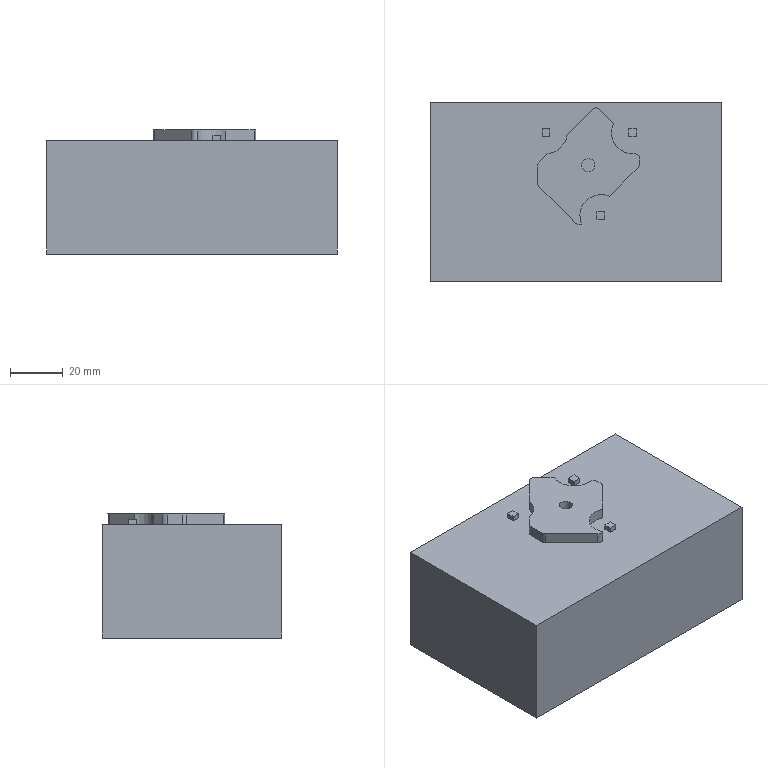NC program | NX | posted with a generic post | part box 110.151 x 68.163 x 47.1 mm
Lines 5088 to 6078 of 32691:
(PLANAR_MILL_2_COPY_COPY_1 , TOOL : D10R0)
N9988 T09 M6
N9990 G54
N9992 G17 G0 G90 X39.075 Y7.328 S4000 M3
N9994 G43 Z80.7 H9
N9996 G94 G1 Z0.7 F5000.
N9998 Y7.828 F800.
N10000 Y18.243
N10002 X29.237 Y28.081
N10004 X-23.529
N10006 X-39.075 Y12.536
N10008 Y-8.293
N10010 X-19.287 Y-28.081
N10012 X33.479
N10014 X43.176 Y-18.385
N10016 X51.308 Y-10.253
N10018 X45.075 Y7.328
N10020 Y7.828
N10022 Y20.728
N10024 X31.722 Y34.081
N10026 X-26.015
N10028 X-45.075 Y15.021
N10030 Y-10.778
N10032 X-21.772 Y-34.081
N10034 X35.964
N10036 X47.419 Y-22.627
N10038 X55.55 Y-14.496
N10040 X51.075 Y7.328
N10042 Y7.828
N10044 Y23.213
N10046 X34.207 Y40.081
N10048 X-28.5
N10050 X-51.075 Y17.506
N10052 Y-13.263
N10054 X-24.257 Y-40.081
N10056 X38.45
N10058 X51.661 Y-26.87
N10060 X59.793 Y-18.738
N10062 G0 Z80.7
N10064 M5
(DRILLING_1 , TOOL : DK-Ø5)
N10066 T01 M6
N10068 G54
N10070 G17 G0 G90 X-77.401 Y70.426 S1500 M3
N10072 G43 Z-44.27 H1
N10074 G94 G81 G99 X-40.278 Y33.303 F150. R-44.27
N10076 G80
N10078 G0 X-77.401 Y70.426 Z-44.27
(DRILLING_1_COPY , TOOL : DK-Ø5)
N10080 X-77.523 Y-74.548 S1800
N10082 G81 X-40.753 Y-37.778 F150. R-44.27
N10084 G80
N10086 G0 X-77.523 Y-74.548 Z-44.27
N10088 M5
(DRILLING_1_COPY_1 , TOOL : D3.7钻头)
N10090 T02 M6
N10092 G54
N10094 G17 G0 G90 X-77.401 Y70.426 S1800 M3
N10096 G43 Z-44.27 H2
N10098 G94 G83 G99 X-27.197 Y20.222 F150. Q5. R-44.27
N10100 G80
N10102 G0 X-77.401 Y70.426 Z-44.27
(DRILLING_1_COPY_COPY , TOOL : D3.7钻头)
N10104 X-77.523 Y-74.548
N10106 G83 X-29.439 Y-26.464 F150. Q5. R-44.27
N10108 G80
N10110 G0 X-77.523 Y-74.548 Z-44.27
N10112 M5
(DRILLING_1_COPY_1_COPY , TOOL : D5.3钻头)
N10114 T03 M6
N10116 G54
N10118 G17 G0 G90 X-77.401 Y70.426 S1500 M3
N10120 G43 Z-44.27 H3
N10122 G94 G81 G99 X-34.975 Y28. F200. R-44.27
N10124 G80
N10126 G0 X-77.401 Y70.426 Z-44.27
N10128 M5
(PLANAR_MILL_3_COPY_3 , TOOL : D8R0)
N10130 T04 M6
N10132 G54
N10134 G17 G0 G90 X-30.025 Y21.975 S5000 M3
N10136 G43 Z30. H4
N10138 G94 G1 Z-15. F3000.
N10140 Y28.775 F1500.
N10142 Y34.5 F1000.
N10144 G2 X-25.975 Y38.55 R4.05
N10146 G1 X16.025
N10148 G2 X20.075 Y34.5 R4.05
N10150 G1 Y28.775
N10152 Y21.975
N10154 G0 Z10.
N10156 X-30.025
N10158 G1 Z-30. F3000.
N10160 Y28.775 F1500.
N10162 Y34.5 F1000.
N10164 G2 X-25.975 Y38.55 R4.05
N10166 G1 X16.025
N10168 G2 X20.075 Y34.5 R4.05
N10170 G1 Y28.775
N10172 Y21.975
N10174 G0 Z10.
N10176 X-30.025
N10178 G1 Z-37.65 F3000.
N10180 Y28.775 F1500.
N10182 Y34.5 F1000.
N10184 G2 X-25.975 Y38.55 R4.05
N10186 G1 X16.025
N10188 G2 X20.075 Y34.5 R4.05
N10190 G1 Y28.775
N10192 Y21.975
N10194 G0 Z30.
(PLANAR_MILL_3_COPY_3_COPY_2 , TOOL : D8R0)
N10196 X-32.466 Y32.637 S5500
N10198 G1 Z-15. F3000.
N10200 X-28.789 Y36.314 F1500.
N10202 X-27.789 Y37.314 F1000.
N10204 X-24.112 Y40.991
N10206 G0 Z10.
N10208 X-32.466 Y32.637
N10210 G1 Z-30. F3000.
N10212 X-28.789 Y36.314 F1500.
N10214 X-27.789 Y37.314 F1000.
N10216 X-24.112 Y40.991
N10218 G0 Z10.
N10220 X-32.466 Y32.637
N10222 G1 Z-37.55 F3000.
N10224 X-28.789 Y36.314 F1500.
N10226 X-27.789 Y37.314 F1000.
N10228 X-24.112 Y40.991
N10230 G0 Z30.
N10232 X14.162
N10234 G1 Z-15. F3000.
N10236 X17.839 Y37.314 F1500.
N10238 X18.839 Y36.314 F1000.
N10240 X22.516 Y32.637
N10242 G0 Z10.
N10244 X14.162 Y40.991
N10246 G1 Z-30. F3000.
N10248 X17.839 Y37.314 F1500.
N10250 X18.839 Y36.314 F1000.
N10252 X22.516 Y32.637
N10254 G0 Z10.
N10256 X14.162 Y40.991
N10258 G1 Z-37.55 F3000.
N10260 X17.839 Y37.314 F1500.
N10262 X18.839 Y36.314 F1000.
N10264 X22.516 Y32.637
N10266 G0 Z30.
(PLANAR_MILL_3_COPY_3_COPY , TOOL : D8R0)
N10268 Z30.242
N10270 X21.225 Y27.289
N10272 G1 Y23.824 Z-9.607 F3000.
N10274 X16.025 F1500.
N10276 X-25.975 F1000.
N10278 X-31.175
N10280 G0 Y25.556 Z10.318
N10282 X21.225
N10284 G1 Y22.957 Z-19.57 F3000.
N10286 X16.025 F1500.
N10288 X-25.975 F1000.
N10290 X-31.175
N10292 G0 Y25.556 Z10.318
N10294 X21.225
N10296 G1 Y22.091 Z-29.532 F3000.
N10298 X16.025 F1500.
N10300 X-25.975 F1000.
N10302 X-31.175
N10304 G0 Y25.556 Z10.318
N10306 X21.225
N10308 G1 Y21.783 Z-33.078 F3000.
N10310 X16.025 F1500.
N10312 X-25.975 F1000.
N10314 X-31.175
N10316 G0 Y27.289 Z30.242
(PLANAR_MILL_3_COPY_3_COPY_COPY_1 , TOOL : D8R0)
N10318 X21.225 Y27.339
N10320 Z30.238
N10322 G1 Y23.873 Z-9.612 F3000.
N10324 X16.025 F1500.
N10326 X-25.975 F1000.
N10328 X-31.175
N10330 G0 Y25.606 Z10.313
N10332 X21.225
N10334 G1 Y23.007 Z-19.574 F3000.
N10336 X16.025 F1500.
N10338 X-25.975 F1000.
N10340 X-31.175
N10342 G0 Y25.606 Z10.313
N10344 X21.225
N10346 G1 Y22.141 Z-29.536 F3000.
N10348 X16.025 F1500.
N10350 X-25.975 F1000.
N10352 X-31.175
N10354 G0 Y25.606 Z10.313
N10356 X21.225
N10358 G1 Y21.832 Z-33.082 F3000.
N10360 X16.025 F1500.
N10362 X-25.975 F1000.
N10364 X-31.175
N10366 G0 Y27.339 Z30.238
(PLANAR_MILL_3_COPY_3_COPY_COPY , TOOL : D8R0)
N10368 X21.225
N10370 G1 Y23.18 Z-17.581 F3000.
N10372 X16.025 F1500.
N10374 X-25.975 F800.
N10376 X-31.175
N10378 G0 Y25.606 Z10.313
N10380 X21.225
N10382 G1 Y21.832 Z-33.082 F3000.
N10384 X16.025 F1500.
N10386 X-25.975 F800.
N10388 X-31.175
N10390 G0 Y27.339 Z30.238
(CAVITY_MILL_COPY_1_COPY , TOOL : D8R0)
N10392 X-32.731 Y47.341
N10394 Z30.15
N10396 G1 Z-38.186 F3000.
N10398 Y42.141 F1500.
N10400 X28.8 F2500.
N10402 X28.843 Y42.123
N10404 X24.83 Y38.111
N10406 G3 X18.882 Y37.395 R4.85
N10408 G1 X18.441 Y36.954
N10410 X17.96 Y37.434
N10412 G3 X17.423 Y37.887 R4.15
N10414 G1 X14.522 Y40.786
N10416 X13.546 Y41.549
N10418 X12.473 Y41.862
N10420 X11.79 Y41.939
N10422 X-15.896 Y41.942
N10424 X-16.395 Y41.935
N10426 X-16.581 Y41.922
N10428 X-17.265 Y41.795
N10430 X-17.948 Y41.542
N10432 X-18.351 Y41.32
N10434 X-18.628 Y41.132
N10436 X-19.183 Y40.634
N10438 X-19.31 Y40.491
N10440 X-19.696 Y39.951
N10442 X-19.994 Y39.344
N10444 X-20.101 Y39.038
N10446 X-20.193 Y38.685
N10448 X-20.219 Y38.65
N10450 X-24.975
N10452 G3 X-27.909 Y37.434 R4.15
N10454 G1 X-30.597 Y34.746
N10456 G3 X-35.338 Y33.506 R4.85
N10458 G1 X-36.646 Y32.198
N10460 X-40.825 Y36.377
N10462 X-36.343 Y40.858
N10464 X-35.078 Y42.124
N10466 X-35.036 Y42.141
N10468 X-32.731
N10470 Y38.541
N10472 X-31.894
N10474 X-31.908 Y38.527
N10476 G3 X-33.798 Y38.313 R8.45
N10478 G1 X-33.569 Y38.541
N10480 X-32.731
N10482 Y43.741
N10484 G0 Z-37.5
N10486 Y47.341
N10488 G1 Z-38.671 F3000.
N10490 Y42.141 F1500.
N10492 X28.8 F2500.
N10494 X28.843 Y42.123
N10496 X24.83 Y38.111
N10498 G3 X18.882 Y37.395 R4.85
N10500 G1 X18.441 Y36.954
N10502 X18.2 Y37.194
N10504 X17.96 Y37.434
N10506 G3 X17.423 Y37.887 R4.15
N10508 G1 X14.522 Y40.786
N10510 X13.546 Y41.549
N10512 X12.473 Y41.862
N10514 X11.79 Y41.939
N10516 X-15.896 Y41.942
N10518 X-16.395 Y41.935
N10520 X-16.581 Y41.922
N10522 X-17.265 Y41.795
N10524 X-17.948 Y41.542
N10526 X-18.351 Y41.32
N10528 X-18.628 Y41.132
N10530 X-19.183 Y40.634
N10532 X-19.31 Y40.491
N10534 X-19.696 Y39.951
N10536 X-19.994 Y39.344
N10538 X-20.101 Y39.038
N10540 X-20.193 Y38.685
N10542 X-20.219 Y38.65
N10544 X-24.975
N10546 G3 X-27.909 Y37.434 R4.15
N10548 G1 X-30.597 Y34.746
N10550 G3 X-35.338 Y33.506 R4.85
N10552 G1 X-36.646 Y32.198
N10554 X-40.825 Y36.377
N10556 X-36.343 Y40.858
N10558 X-35.078 Y42.124
N10560 X-35.036 Y42.141
N10562 X-32.731
N10564 Y38.541
N10566 X-31.894
N10568 X-31.908 Y38.527
N10570 G3 X-33.798 Y38.313 R8.45
N10572 G1 X-33.569 Y38.541
N10574 X-32.731
N10576 Y43.741
N10578 G0 Z-37.986
N10580 Y47.341
N10582 G1 Z-39.157 F3000.
N10584 Y42.141 F1500.
N10586 X28.8 F2500.
N10588 X28.843 Y42.123
N10590 X24.83 Y38.111
N10592 G3 X18.882 Y37.395 R4.85
N10594 G1 X18.441 Y36.954
N10596 X17.96 Y37.434
N10598 G3 X17.423 Y37.887 R4.15
N10600 G1 X14.522 Y40.786
N10602 X13.546 Y41.549
N10604 X12.473 Y41.862
N10606 X11.79 Y41.939
N10608 X-15.896 Y41.942
N10610 X-16.395 Y41.935
N10612 X-16.581 Y41.922
N10614 X-17.265 Y41.795
N10616 X-17.948 Y41.542
N10618 X-18.351 Y41.32
N10620 X-18.628 Y41.132
N10622 X-19.183 Y40.634
N10624 X-19.31 Y40.491
N10626 X-19.696 Y39.951
N10628 X-19.994 Y39.344
N10630 X-20.101 Y39.038
N10632 X-20.193 Y38.685
N10634 X-20.219 Y38.65
N10636 X-24.975
N10638 G3 X-27.909 Y37.434 R4.15
N10640 G1 X-30.597 Y34.746
N10642 G3 X-35.338 Y33.506 R4.85
N10644 G1 X-36.646 Y32.198
N10646 X-40.825 Y36.377
N10648 X-36.343 Y40.858
N10650 X-35.078 Y42.124
N10652 X-35.036 Y42.141
N10654 X-32.731
N10656 Y38.541
N10658 X-31.894
N10660 X-31.908 Y38.527
N10662 G3 X-33.798 Y38.313 R8.45
N10664 G1 X-33.569 Y38.541
N10666 X-32.731
N10668 Y43.741
N10670 G0 Z-38.471
N10672 Y47.341
N10674 G1 Z-39.643 F3000.
N10676 Y42.141 F1500.
N10678 X28.8 F2500.
N10680 X28.843 Y42.123
N10682 X24.83 Y38.111
N10684 G3 X18.882 Y37.395 R4.85
N10686 G1 X18.441 Y36.954
N10688 X17.96 Y37.434
N10690 G3 X17.423 Y37.887 R4.15
N10692 G1 X14.522 Y40.786
N10694 X13.546 Y41.549
N10696 X12.473 Y41.862
N10698 X11.79 Y41.939
N10700 X-15.896 Y41.942
N10702 X-16.395 Y41.935
N10704 X-16.581 Y41.922
N10706 X-17.265 Y41.795
N10708 X-17.948 Y41.542
N10710 X-18.351 Y41.32
N10712 X-18.628 Y41.132
N10714 X-19.183 Y40.634
N10716 X-19.31 Y40.491
N10718 X-19.696 Y39.951
N10720 X-19.994 Y39.344
N10722 X-20.101 Y39.038
N10724 X-20.193 Y38.685
N10726 X-20.219 Y38.65
N10728 X-24.975
N10730 G3 X-27.909 Y37.434 R4.15
N10732 G1 X-30.597 Y34.746
N10734 G3 X-35.338 Y33.506 R4.85
N10736 G1 X-36.646 Y32.198
N10738 X-40.825 Y36.377
N10740 X-36.343 Y40.858
N10742 X-35.078 Y42.124
N10744 X-35.036 Y42.141
N10746 X-32.731
N10748 Y38.541
N10750 X-31.894
N10752 X-31.908 Y38.527
N10754 G3 X-33.798 Y38.313 R8.45
N10756 G1 X-33.569 Y38.541
N10758 X-32.731
N10760 Y43.741
N10762 G0 Z-38.957
N10764 Y47.341
N10766 G1 Z-40.129 F3000.
N10768 Y42.141 F1500.
N10770 X28.8 F2500.
N10772 X28.843 Y42.123
N10774 X24.83 Y38.111
N10776 G3 X18.882 Y37.395 R4.85
N10778 G1 X18.441 Y36.954
N10780 X17.697 Y37.697
N10782 G3 X17.146 Y38.164 R4.24
N10784 G1 X14.522 Y40.786
N10786 X13.546 Y41.549
N10788 X12.473 Y41.862
N10790 X11.79 Y41.939
N10792 X-15.896 Y41.942
N10794 X-16.395 Y41.935
N10796 X-16.581 Y41.922
N10798 X-17.265 Y41.795
N10800 X-17.948 Y41.542
N10802 X-18.351 Y41.32
N10804 X-18.628 Y41.132
N10806 X-19.183 Y40.634
N10808 X-19.31 Y40.491
N10810 X-19.696 Y39.951
N10812 X-19.994 Y39.344
N10814 X-20.101 Y39.038
N10816 X-20.189 Y38.7
N10818 X-24.925
N10820 G3 X-27.859 Y37.484 R4.15
N10822 G1 X-30.597 Y34.746
N10824 G3 X-35.338 Y33.506 R4.85
N10826 G1 X-36.646 Y32.198
N10828 X-40.825 Y36.377
N10830 X-36.343 Y40.858
N10832 X-35.078 Y42.124
N10834 X-35.036 Y42.141
N10836 X-32.731
N10838 Y38.541
N10840 X-31.894
N10842 X-31.908 Y38.527
N10844 G3 X-33.798 Y38.313 R8.45
N10846 G1 X-33.569 Y38.541
N10848 X-32.731
N10850 Y43.741
N10852 G0 Z-39.443
N10854 Y47.341
N10856 G1 Z-40.614 F3000.
N10858 Y42.141 F1500.
N10860 X28.8 F2500.
N10862 X28.843 Y42.123
N10864 X24.83 Y38.111
N10866 G3 X18.882 Y37.395 R4.85
N10868 G1 X18.441 Y36.954
N10870 X17.258 Y38.136
N10872 G3 X16.707 Y38.603 R4.24
N10874 G1 X14.522 Y40.786
N10876 X13.546 Y41.549
N10878 X12.473 Y41.862
N10880 X11.79 Y41.939
N10882 X-15.896 Y41.942
N10884 X-16.395 Y41.935
N10886 X-16.581 Y41.922
N10888 X-17.265 Y41.795
N10890 X-17.948 Y41.542
N10892 X-18.351 Y41.32
N10894 X-18.628 Y41.132
N10896 X-19.183 Y40.634
N10898 X-19.31 Y40.491
N10900 X-19.696 Y39.951
N10902 X-19.994 Y39.344
N10904 X-20.101 Y39.038
N10906 X-20.189 Y38.7
N10908 X-24.925
N10910 G3 X-27.859 Y37.484 R4.15
N10912 G1 X-30.597 Y34.746
N10914 G3 X-35.338 Y33.506 R4.85
N10916 G1 X-36.646 Y32.198
N10918 X-40.825 Y36.377
N10920 X-36.343 Y40.858
N10922 X-35.078 Y42.124
N10924 X-35.036 Y42.141
N10926 X-32.731
N10928 Y38.541
N10930 X-31.894
N10932 X-31.908 Y38.527
N10934 G3 X-33.798 Y38.313 R8.45
N10936 G1 X-33.569 Y38.541
N10938 X-32.731
N10940 Y43.741
N10942 G0 Z-39.929
N10944 Y47.341
N10946 G1 Z-41.1 F3000.
N10948 Y42.141 F1500.
N10950 X28.8 F2500.
N10952 X28.843 Y42.123
N10954 X24.83 Y38.111
N10956 G3 X18.882 Y37.395 R4.85
N10958 G1 X18.441 Y36.954
N10960 X17.242 Y38.152
N10962 X16.819 Y38.575
N10964 G3 X16.267 Y39.042 R4.24
N10966 G1 X14.522 Y40.786
N10968 X13.546 Y41.549
N10970 X12.473 Y41.862
N10972 X11.79 Y41.939
N10974 X-15.896 Y41.942
N10976 X-16.395 Y41.935
N10978 X-16.581 Y41.922
N10980 X-17.265 Y41.795
N10982 X-17.948 Y41.542
N10984 X-18.351 Y41.32
N10986 X-18.628 Y41.132
N10988 X-19.183 Y40.634
N10990 X-19.31 Y40.491
N10992 X-19.696 Y39.951
N10994 X-19.994 Y39.344
N10996 X-20.101 Y39.038
N10998 X-20.189 Y38.701
N11000 X-24.925 Y38.7
N11002 G3 X-27.859 Y37.484 R4.15
N11004 G1 X-30.597 Y34.746
N11006 G3 X-35.338 Y33.506 R4.85
N11008 G1 X-36.646 Y32.198
N11010 X-40.825 Y36.377
N11012 X-36.343 Y40.858
N11014 X-35.078 Y42.124
N11016 X-35.036 Y42.141
N11018 X-32.731
N11020 Y38.541
N11022 X-31.894
N11024 X-31.908 Y38.527
N11026 G3 X-33.798 Y38.313 R8.45
N11028 G1 X-33.569 Y38.541
N11030 X-32.731
N11032 Y43.741
N11034 G0 Z-40.414
N11036 Y47.341
N11038 G1 Z-41.586 F3000.
N11040 Y42.141 F1500.
N11042 X28.8 F2500.
N11044 X28.843 Y42.123
N11046 X24.83 Y38.111
N11048 G3 X18.882 Y37.395 R4.85
N11050 G1 X18.441 Y36.954
N11052 X16.381 Y39.013
N11054 G3 X15.865 Y39.445 R4.407
N11056 G1 X14.522 Y40.786
N11058 X13.546 Y41.549
N11060 X12.473 Y41.862
N11062 X11.79 Y41.939
N11064 X-15.896 Y41.942
N11066 X-16.395 Y41.935
N11068 X-16.581 Y41.922
N11070 X-17.265 Y41.795
N11072 X-17.948 Y41.542
N11074 X-18.351 Y41.32
N11076 X-18.628 Y41.132
N11078 X-19.183 Y40.634
N11080 X-19.31 Y40.491
N11082 X-19.696 Y39.951
N11084 X-19.994 Y39.344
N11086 X-20.101 Y39.038
N11088 X-20.185 Y38.717
N11090 X-20.198 Y38.7
N11092 X-24.925
N11094 G3 X-27.859 Y37.484 R4.15
N11096 G1 X-30.597 Y34.746
N11098 G3 X-35.338 Y33.506 R4.85
N11100 G1 X-36.646 Y32.198
N11102 X-40.825 Y36.377
N11104 X-36.343 Y40.858
N11106 X-35.078 Y42.124
N11108 X-35.036 Y42.141
N11110 X-32.731
N11112 Y38.541
N11114 X-31.894
N11116 X-31.908 Y38.527
N11118 G3 X-33.798 Y38.313 R8.45
N11120 G1 X-33.569 Y38.541
N11122 X-32.731
N11124 Y43.741
N11126 G0 Z-40.9
N11128 Y47.341
N11130 G1 Z-42.071 F3000.
N11132 Y42.141 F1500.
N11134 X28.8 F2500.
N11136 X28.843 Y42.123
N11138 X24.83 Y38.111
N11140 G3 X18.882 Y37.395 R4.85
N11142 G1 X18.441 Y36.954
N11144 X15.942 Y39.452
N11146 G3 X15.388 Y39.921 R4.24
N11148 G1 X14.522 Y40.786
N11150 X13.546 Y41.549
N11152 X12.473 Y41.862
N11154 X11.79 Y41.939
N11156 X-15.896 Y41.942
N11158 X-16.395 Y41.935
N11160 X-16.581 Y41.922
N11162 X-17.265 Y41.795
N11164 X-17.948 Y41.542
N11166 X-18.351 Y41.32
N11168 X-18.628 Y41.132
N11170 X-19.183 Y40.634
N11172 X-19.31 Y40.491
N11174 X-19.696 Y39.951
N11176 X-19.994 Y39.344
N11178 X-20.101 Y39.038
N11180 X-20.178 Y38.742
N11182 X-20.204 Y38.7
N11184 X-24.925
N11186 G3 X-27.859 Y37.484 R4.15
N11188 G1 X-30.597 Y34.746
N11190 G3 X-35.338 Y33.506 R4.85
N11192 G1 X-36.646 Y32.198
N11194 X-40.825 Y36.377
N11196 X-36.343 Y40.858
N11198 X-35.078 Y42.124
N11200 X-35.036 Y42.141
N11202 X-32.731
N11204 Y38.541
N11206 X-31.894
N11208 X-31.908 Y38.527
N11210 G3 X-33.798 Y38.313 R8.45
N11212 G1 X-33.569 Y38.541
N11214 X-32.731
N11216 Y43.741
N11218 G0 Z-41.386
N11220 Y47.341
N11222 G1 Z-42.557 F3000.
N11224 Y42.141 F1500.
N11226 X28.8 F2500.
N11228 X28.843 Y42.123
N11230 X24.83 Y38.111
N11232 G3 X18.882 Y37.395 R4.85
N11234 G1 X18.441 Y36.954
N11236 X15.503 Y39.891
N11238 G3 X14.948 Y40.36 R4.24
N11240 G1 X14.522 Y40.786
N11242 X13.546 Y41.549
N11244 X12.473 Y41.862
N11246 X11.79 Y41.939
N11248 X-15.896 Y41.942
N11250 X-16.395 Y41.935
N11252 X-16.581 Y41.922
N11254 X-17.265 Y41.795
N11256 X-17.948 Y41.542
N11258 X-18.351 Y41.32
N11260 X-18.628 Y41.132
N11262 X-19.183 Y40.634
N11264 X-19.31 Y40.491
N11266 X-19.696 Y39.951
N11268 X-19.994 Y39.344
N11270 X-20.101 Y39.038
N11272 X-20.155 Y38.83
N11274 X-20.216 Y38.7
N11276 X-24.925
N11278 G3 X-27.859 Y37.484 R4.15
N11280 G1 X-30.597 Y34.746
N11282 G3 X-35.338 Y33.506 R4.85
N11284 G1 X-36.646 Y32.198
N11286 X-40.825 Y36.377
N11288 X-36.343 Y40.858
N11290 X-35.078 Y42.124
N11292 X-35.036 Y42.141
N11294 X-32.731
N11296 Y38.541
N11298 X-31.894
N11300 X-31.908 Y38.527
N11302 G3 X-33.798 Y38.313 R8.45
N11304 G1 X-33.569 Y38.541
N11306 X-32.731
N11308 Y43.741
N11310 G0 Z-41.871
N11312 Y47.341
N11314 G1 Z-43.043 F3000.
N11316 Y42.141 F1500.
N11318 X28.8 F2500.
N11320 X28.843 Y42.123
N11322 X24.83 Y38.111
N11324 G3 X18.882 Y37.395 R4.85
N11326 G1 X18.441 Y36.954
N11328 X15.065 Y40.33
N11330 G3 X14.473 Y40.825 R4.24
N11332 G1 X13.546 Y41.549
N11334 X12.473 Y41.862
N11336 X11.79 Y41.939
N11338 X-15.896 Y41.942
N11340 X-16.395 Y41.935
N11342 X-16.581 Y41.922
N11344 X-17.265 Y41.795
N11346 X-17.948 Y41.542
N11348 X-18.351 Y41.32
N11350 X-18.628 Y41.132
N11352 X-19.183 Y40.634
N11354 X-19.31 Y40.491
N11356 X-19.696 Y39.951
N11358 X-19.994 Y39.344
N11360 X-20.083 Y39.088
N11362 G3 X-20.23 Y38.7 R4.146
N11364 G1 X-24.925
N11366 G3 X-27.859 Y37.484 R4.15
N11368 G1 X-30.597 Y34.746
N11370 G3 X-35.338 Y33.506 R4.85
N11372 G1 X-36.646 Y32.198
N11374 X-40.825 Y36.377
N11376 X-36.343 Y40.858
N11378 X-35.078 Y42.124
N11380 X-35.036 Y42.141
N11382 X-32.731
N11384 Y38.541
N11386 X-31.894
N11388 X-31.908 Y38.527
N11390 G3 X-33.798 Y38.313 R8.45
N11392 G1 X-33.569 Y38.541
N11394 X-32.731
N11396 Y43.741
N11398 G0 Z-42.357
N11400 Y47.341
N11402 G1 Z-43.529 F3000.
N11404 Y42.141 F1500.
N11406 X28.8 F2500.
N11408 X28.843 Y42.123
N11410 X24.83 Y38.111
N11412 G3 X18.882 Y37.395 R4.85
N11414 G1 X18.441 Y36.954
N11416 X14.626 Y40.768
N11418 G3 X11.703 Y41.998 R4.143
N11420 G1 X-16.159
N11422 G3 X-20.248 Y38.7 R4.152
N11424 G1 X-24.925
N11426 G3 X-27.859 Y37.484 R4.15
N11428 G1 X-30.597 Y34.746
N11430 G3 X-35.338 Y33.506 R4.85
N11432 G1 X-36.646 Y32.198
N11434 X-40.825 Y36.377
N11436 X-36.343 Y40.858
N11438 X-35.078 Y42.124
N11440 X-35.036 Y42.141
N11442 X-32.731
N11444 Y38.541
N11446 X-31.894
N11448 X-31.908 Y38.527
N11450 G3 X-33.798 Y38.313 R8.45
N11452 G1 X-33.569 Y38.541
N11454 X-32.731
N11456 Y43.741
N11458 G0 Z-42.843
N11460 Y47.341
N11462 G1 Z-44.014 F3000.
N11464 Y42.141 F1500.
N11466 X28.8 F2500.
N11468 X28.843 Y42.123
N11470 X24.83 Y38.111
N11472 G3 X18.882 Y37.395 R4.85
N11474 G1 X18.441 Y36.954
N11476 X14.626 Y40.768
N11478 G3 X13.877 Y41.368 R4.143
N11480 X11.675 Y42. R4.15
N11482 G1 X-16.187
N11484 G3 X-20.249 Y38.7 R4.15
N11486 G1 X-24.925
N11488 G3 X-27.859 Y37.484 R4.15
N11490 G1 X-30.597 Y34.746
N11492 G3 X-35.338 Y33.506 R4.85
N11494 G1 X-36.646 Y32.198
N11496 X-40.825 Y36.377
N11498 X-36.343 Y40.858
N11500 X-35.078 Y42.124
N11502 X-35.036 Y42.141
N11504 X-32.731
N11506 Y38.541
N11508 X-31.894
N11510 X-31.908 Y38.527
N11512 G3 X-33.798 Y38.313 R8.45
N11514 G1 X-33.569 Y38.541
N11516 X-32.731
N11518 Y43.741
N11520 G0 Z-43.329
N11522 Y47.341
N11524 G1 Z-44.5 F3000.
N11526 Y42.141 F1500.
N11528 X28.8 F2500.
N11530 X28.843 Y42.123
N11532 X24.83 Y38.111
N11534 G3 X18.882 Y37.395 R4.85
N11536 G1 X18.441 Y36.954
N11538 X14.626 Y40.768
N11540 G3 X13.877 Y41.368 R4.143
N11542 X11.675 Y42. R4.15
N11544 G1 X-16.187
N11546 G3 X-20.249 Y38.7 R4.15
N11548 G1 X-24.925
N11550 G3 X-27.859 Y37.484 R4.15
N11552 G1 X-30.597 Y34.746
N11554 G3 X-35.338 Y33.506 R4.85
N11556 G1 X-36.646 Y32.198
N11558 X-40.825 Y36.377
N11560 X-36.343 Y40.858
N11562 X-35.078 Y42.124
N11564 X-35.036 Y42.141
N11566 X-32.731
N11568 Y38.541
N11570 X-31.894
N11572 X-31.908 Y38.527
N11574 G3 X-33.798 Y38.313 R8.45
N11576 G1 X-33.569 Y38.541
N11578 X-32.731
N11580 Y43.741
N11582 G0 Z30.15
(PLANAR_PROFILE_COPY , TOOL : D8R0)
N11584 X-41.317 Y43.851
N11586 Z-7.
N11588 G1 Z-44.6 F5000.
N11590 G41 X-41.03 Y43.441 F1500. D4
N11592 X-37.353 Y39.764
N11594 X-36.309 Y38.721 F1000.
N11596 G2 X-32.441 Y39.762 R9.7
N11598 G1 X-31.289 Y40.914
N11600 G2 X-24.925 Y43.55 R9.
N11602 G1 X-23.152
N11604 G2 X-16.187 Y46.85 R9.
N11606 G1 X11.675
N11608 G2 X18.039 Y44.214 R9.
N11610 G1 X19.125 Y43.128
N11612 G2 X23.459 Y43.598 R9.7
N11614 G1 X25.635 Y45.775
N11616 X29.312 Y49.452
N11618 G40
N11620 X29.599 Y49.861
N11622 G0 Z-7.
(PLANAR_PROFILE_COPY_COPY , TOOL : D8R0)
N11624 X-44.746 Y40.421
N11626 G1 Z-44.6 F5000.
N11628 G41 X-44.459 Y40.012 F1500.
N11630 X-40.782 Y36.335
N11632 X-36.646 Y32.198 F650.
N11634 X-35.338 Y33.506
N11636 G2 X-30.597 Y34.746 R4.85
N11638 G1 X-27.859 Y37.484
N11640 G2 X-24.925 Y38.7 R4.15
N11642 G1 X-20.249
N11644 G2 X-16.187 Y42. R4.15
N11646 G1 X11.675
N11648 G2 X14.61 Y40.784 R4.15
N11650 G1 X18.441 Y36.954
N11652 X18.882 Y37.395
N11654 G2 X24.83 Y38.111 R4.85
N11656 G1 X29.065 Y42.345
N11658 X32.742 Y46.022
N11660 G40
N11662 X33.028 Y46.432
N11664 G0 Z-7.
N11666 M5
(PLANAR_MILL_4 , TOOL : D6R0)
N11668 T05 M6
N11670 G54
N11672 G17 G0 G90 X18.983 Y98.777 S6500 M3
N11674 G43 Z14.318 H5
N11676 G94 G1 Y39.04 Z-39.642 F5000.
N11678 X16.583 F2500.
N11680 X-25.817
N11682 Y38.118 Z-38.621
N11684 X16.083
N11686 X18.483
N11688 G0 X18.983 Y38.669 Z-39.977
N11690 G1 X16.583
N11692 X-25.817
N11694 Y37.746 Z-38.956
N11696 X16.083
N11698 X18.483
N11700 G0 X18.983 Y38.298 Z-40.312
N11702 G1 X16.583
N11704 X-25.817
N11706 Y37.375 Z-39.291
N11708 X16.083
N11710 X18.483
N11712 G0 X18.983 Y37.927 Z-40.647
N11714 G1 X16.583
N11716 X-25.817
N11718 Y37.004 Z-39.627
N11720 X16.083
N11722 X18.483
N11724 G0 X18.983 Y37.555 Z-40.983
N11726 G1 X16.583
N11728 X-25.817
N11730 Y36.633 Z-39.962
N11732 X16.083
N11734 X18.483
N11736 G0 X18.983 Y37.184 Z-41.318
N11738 G1 X16.583
N11740 X-25.817
N11742 Y36.262 Z-40.297
N11744 X16.083
N11746 X18.483
N11748 G0 X18.983 Y36.813 Z-41.653
N11750 G1 X16.583
N11752 X-25.817
N11754 Y35.891 Z-40.632
N11756 X16.083
N11758 X18.483
N11760 G0 X18.983 Y36.517 Z-41.921
N11762 G1 X16.583
N11764 X-25.817
N11766 Y35.594 Z-40.9
N11768 X16.083
N11770 X18.483
N11772 G0 Y97.855 Z15.339
(PLANAR_MILL_4_COPY , TOOL : D6R0)
N11774 X18.983 Y98.844
N11776 Z14.244
N11778 G1 Y36.509 Z-42.062 F5000.
N11780 X16.583 F800.
N11782 X-25.917
N11784 Y35.453 Z-40.893
N11786 X16.083
N11788 X18.483
N11790 G0 Y97.788 Z15.413
N11792 M5
(PLANAR_MILL_3_COPY_3_COPY_COPY_COPY_COPY , TOOL : D10)
N11794 T12 M6
N11796 G54
N11798 G17 G0 G90 X22.525 Y26.392 S3000 M3
N11800 G43 Z30.32 H12
N11802 G94 G1 Y20.886 Z-33. F3000.
N11804 X16.025 F1500.
N11806 X-25.975 F800.
N11808 X-32.475
N11810 G0 Y26.392 Z30.32
(PLANAR_MILL_3_COPY_3_COPY_1 , TOOL : D10)
N11812 X-30.975 Y20.275 S5000
N11814 Z30.
N11816 G1 Z-37.65 F3000.
N11818 Y28.775 F1500.
N11820 Y34.5 F1000.
N11822 G2 X-25.975 Y39.5 R5.
N11824 G1 X16.025
N11826 G2 X21.025 Y34.5 R5.
N11828 G1 Y28.775
N11830 Y20.275
N11832 G0 Z30.
(PLANAR_MILL_3_COPY_3_COPY_1_COPY_1 , TOOL : D10)
N11834 X-30.975
N11836 G1 Z-37.65 F3000.
N11838 Y28.775 F1500.
N11840 Y34.5 F1000.
N11842 G2 X-25.975 Y39.5 R5.
N11844 G1 X16.025
N11846 G2 X21.025 Y34.5 R5.
N11848 G1 Y28.775
N11850 Y20.275
N11852 G0 Z30.
N11854 M5